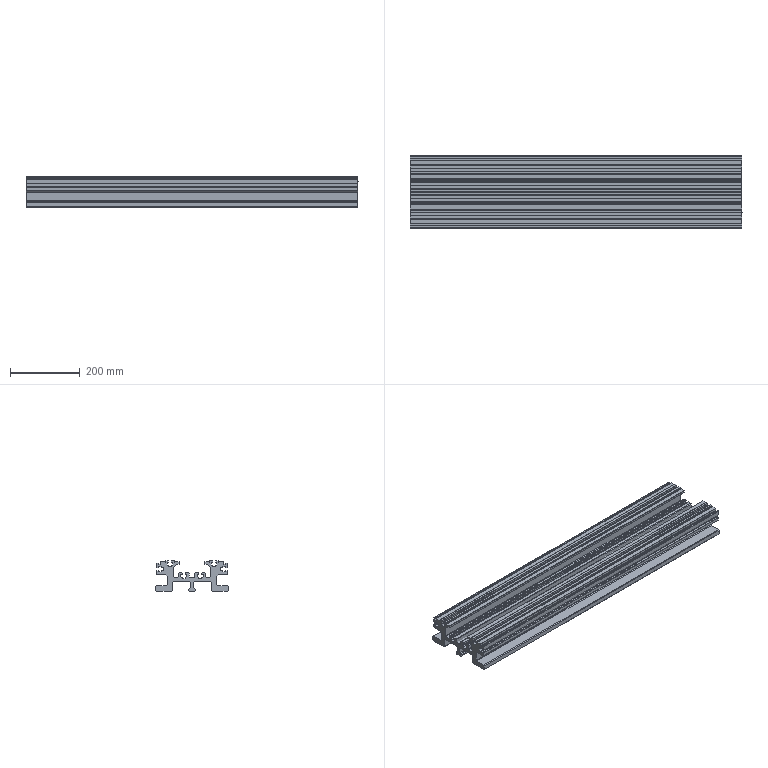Part | NX | features DATUM_CSYS 1, EXTRUDE 1 | 1 solid | 210 faces | box 950 x 207.383 x 87 mm | volume 7328516 mm3 | plane 190 | spline 20